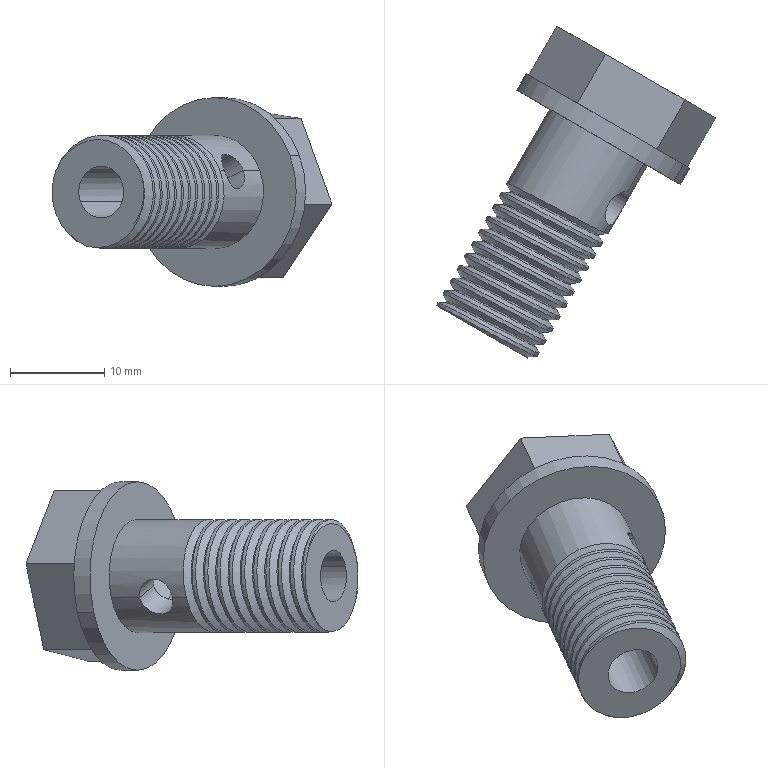Part | SolidWorks | features BaseBody 1 | 1 solid | 46 faces | box 29.624 x 35.187 x 20 mm | volume 4063 mm3 | cylinder 30 | plane 11 | spline 3 | cone 2 | commonest cylinder face diameters 12 x22 4 x4 5.5 x2 20 x2